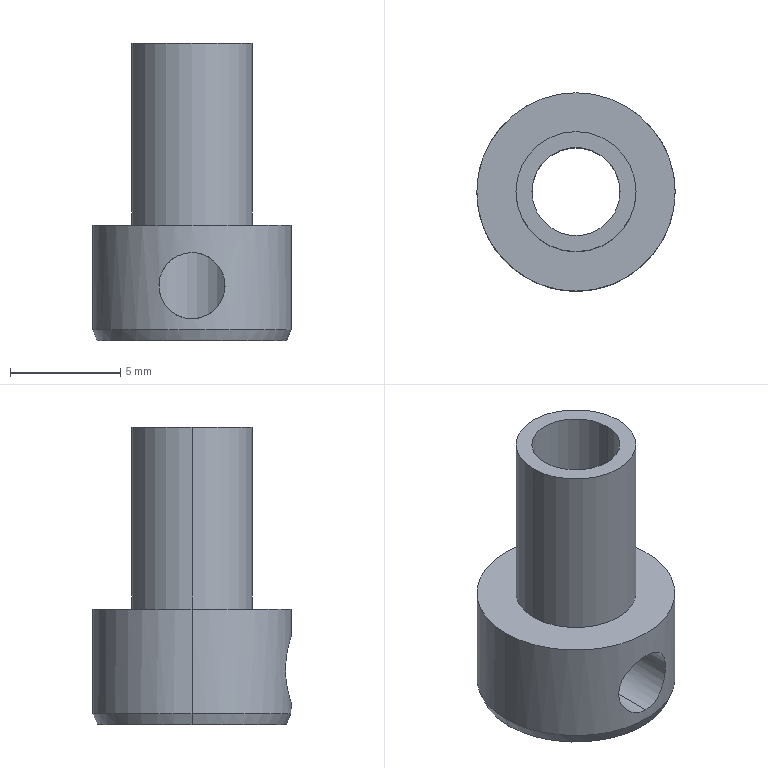Part | SolidWorks | features ICE 3, Blend 1, Extrusion 1 | 1 solid | 13 faces | box 9 x 9 x 13.5 mm | volume 337.082 mm3 | cylinder 8 | plane 3 | spline 2 | commonest cylinder face diameters 3 x2 4 x2 5.45 x2 9 x2
STEP:
#1=CARTESIAN_POINT('',(0.,-4.5,3.5));
#2=VERTEX_POINT('',#1);
#3=CARTESIAN_POINT('',(0.,-4.5,0.5));
#4=VERTEX_POINT('',#3);
#5=CARTESIAN_POINT('',(0.,-4.5,3.5));
#6=CARTESIAN_POINT('',(-0.09988,-4.5,3.5));
#7=CARTESIAN_POINT('',(-0.198,-4.497,3.49));
#8=CARTESIAN_POINT('',(-0.3907,-4.484,3.452));
#9=CARTESIAN_POINT('',(-0.4864,-4.475,3.422));
#10=CARTESIAN_POINT('',(-0.7584,-4.439,3.309));
#11=CARTESIAN_POINT('',(-0.9239,-4.406,3.198));
#12=CARTESIAN_POINT('',(-1.198,-4.34,2.923));
#13=CARTESIAN_POINT('',(-1.31,-4.306,2.757));
#14=CARTESIAN_POINT('',(-1.46,-4.257,2.396));
#15=CARTESIAN_POINT('',(-1.5,-4.243,2.198));
#16=CARTESIAN_POINT('',(-1.5,-4.243,1.902));
#17=CARTESIAN_POINT('',(-1.49,-4.246,1.802));
#18=CARTESIAN_POINT('',(-1.451,-4.26,1.609));
#19=CARTESIAN_POINT('',(-1.423,-4.269,1.515));
#20=CARTESIAN_POINT('',(-1.309,-4.306,1.241));
#21=CARTESIAN_POINT('',(-1.198,-4.34,1.077));
#22=CARTESIAN_POINT('',(-0.9912,-4.39,0.8699));
#23=CARTESIAN_POINT('',(-0.9162,-4.407,0.8083));
#24=CARTESIAN_POINT('',(-0.7541,-4.437,0.6997));
#25=CARTESIAN_POINT('',(-0.6663,-4.451,0.6526));
#26=CARTESIAN_POINT('',(-0.3954,-4.486,0.5399));
#27=CARTESIAN_POINT('',(-0.1968,-4.5,0.5));
#28=CARTESIAN_POINT('',(0.,-4.5,0.5));
#29=B_SPLINE_CURVE_WITH_KNOTS('',3,(#5,#6,#7,#8,#9,#10,#11,#12,#13,#14,#15,#16,#17,#18,#19,#20,#21,#22,#23,#24,#25,#26,#27,#28),.UNSPECIFIED.,.F.,.F.,(4,2,2,2,2,2,2,2,2,2,2,4),(0.,0.0002952,0.0005905,0.001181,0.001771,0.002362,0.002657,0.002952,0.003543,0.003838,0.004133,0.004724),.UNSPECIFIED.);
#30=EDGE_CURVE('',#2,#4,#29,.T.);
#31=ORIENTED_EDGE('',*,*,#30,.T.);
#32=CARTESIAN_POINT('',(0.,-2.,0.5));
#33=VERTEX_POINT('',#32);
#34=CARTESIAN_POINT('',(0.,-4.501,0.5));
#35=DIRECTION('',(0.,1.,0.));
#36=VECTOR('',#35,1000.);
#37=LINE('',#34,#36);
#38=EDGE_CURVE('',#4,#33,#37,.T.);
#39=ORIENTED_EDGE('',*,*,#38,.T.);
#40=CARTESIAN_POINT('',(0.,-2.,3.5));
#41=VERTEX_POINT('',#40);
#42=CARTESIAN_POINT('',(0.,-2.,0.5));
#43=CARTESIAN_POINT('',(-0.1025,-2.,0.5));
#44=CARTESIAN_POINT('',(-0.2067,-1.992,0.5108));
#45=CARTESIAN_POINT('',(-0.4052,-1.961,0.5522));
#46=CARTESIAN_POINT('',(-0.5023,-1.938,0.5831));
#47=CARTESIAN_POINT('',(-0.7754,-1.853,0.7007));
#48=CARTESIAN_POINT('',(-0.9353,-1.775,0.8124));
#49=CARTESIAN_POINT('',(-1.199,-1.608,1.079));
#50=CARTESIAN_POINT('',(-1.305,-1.519,1.237));
#51=CARTESIAN_POINT('',(-1.455,-1.376,1.589));
#52=CARTESIAN_POINT('',(-1.5,-1.323,1.794));
#53=CARTESIAN_POINT('',(-1.5,-1.323,2.207));
#54=CARTESIAN_POINT('',(-1.456,-1.375,2.409));
#55=CARTESIAN_POINT('',(-1.343,-1.483,2.675));
#56=CARTESIAN_POINT('',(-1.297,-1.524,2.759));
#57=CARTESIAN_POINT('',(-1.192,-1.607,2.915));
#58=CARTESIAN_POINT('',(-1.133,-1.65,2.987));
#59=CARTESIAN_POINT('',(-1.001,-1.733,3.121));
#60=CARTESIAN_POINT('',(-0.9275,-1.774,3.183));
#61=CARTESIAN_POINT('',(-0.7704,-1.848,3.291));
#62=CARTESIAN_POINT('',(-0.6862,-1.881,3.338));
#63=CARTESIAN_POINT('',(-0.4131,-1.966,3.456));
#64=CARTESIAN_POINT('',(-0.2077,-2.,3.5));
#65=CARTESIAN_POINT('',(0.,-2.,3.5));
#66=B_SPLINE_CURVE_WITH_KNOTS('',3,(#42,#43,#44,#45,#46,#47,#48,#49,#50,#51,#52,#53,#54,#55,#56,#57,#58,#59,#60,#61,#62,#63,#64,#65),.UNSPECIFIED.,.F.,.F.,(4,2,2,2,2,2,2,2,2,2,2,4),(0.004913,0.005219,0.005526,0.006139,0.006751,0.007364,0.007977,0.008283,0.00859,0.008896,0.009203,0.009816),.UNSPECIFIED.);
#67=EDGE_CURVE('',#33,#41,#66,.T.);
#68=ORIENTED_EDGE('',*,*,#67,.T.);
#69=CARTESIAN_POINT('',(0.,-4.501,3.5));
#70=DIRECTION('',(0.,1.,0.));
#71=VECTOR('',#70,1000.);
#72=LINE('',#69,#71);
#73=EDGE_CURVE('',#2,#41,#72,.T.);
#74=ORIENTED_EDGE('',*,*,#73,.F.);
#75=EDGE_LOOP('',(#31,#39,#68,#74));
#76=FACE_OUTER_BOUND('',#75,.T.);
#77=CARTESIAN_POINT('',(0.,-4.501,2.));
#78=DIRECTION('',(0.,1.,0.));
#79=DIRECTION('',(0.,0.,1.));
#80=AXIS2_PLACEMENT_3D('',#77,#78,#79);
#81=CYLINDRICAL_SURFACE('',#80,1.5);
#82=ADVANCED_FACE('',(#76),#81,.F.);
#83=CARTESIAN_POINT('',(0.,-2.,3.5));
#84=CARTESIAN_POINT('',(0.104,-2.,3.5));
#85=CARTESIAN_POINT('',(0.2056,-1.992,3.489));
#86=CARTESIAN_POINT('',(0.4043,-1.961,3.448));
#87=CARTESIAN_POINT('',(0.5019,-1.938,3.417));
#88=CARTESIAN_POINT('',(0.7741,-1.854,3.3));
#89=CARTESIAN_POINT('',(0.9344,-1.775,3.188));
#90=CARTESIAN_POINT('',(1.199,-1.608,2.921));
#91=CARTESIAN_POINT('',(1.305,-1.519,2.765));
#92=CARTESIAN_POINT('',(1.418,-1.411,2.498));
#93=CARTESIAN_POINT('',(1.448,-1.38,2.403));
#94=CARTESIAN_POINT('',(1.489,-1.335,2.207));
#95=CARTESIAN_POINT('',(1.5,-1.323,2.102));
#96=CARTESIAN_POINT('',(1.5,-1.323,1.898));
#97=CARTESIAN_POINT('',(1.489,-1.335,1.794));
#98=CARTESIAN_POINT('',(1.448,-1.38,1.596));
#99=CARTESIAN_POINT('',(1.418,-1.411,1.502));
#100=CARTESIAN_POINT('',(1.342,-1.484,1.324));
#101=CARTESIAN_POINT('',(1.297,-1.524,1.241));
#102=CARTESIAN_POINT('',(1.192,-1.607,1.085));
#103=CARTESIAN_POINT('',(1.132,-1.651,1.012));
#104=CARTESIAN_POINT('',(0.9999,-1.734,0.878));
#105=CARTESIAN_POINT('',(0.9277,-1.774,0.8174));
#106=CARTESIAN_POINT('',(0.7696,-1.848,0.7089));
#107=CARTESIAN_POINT('',(0.683,-1.882,0.6609));
#108=CARTESIAN_POINT('',(0.4107,-1.967,0.5438));
#109=CARTESIAN_POINT('',(0.2055,-2.,0.5));
#110=CARTESIAN_POINT('',(0.,-2.,0.5));
#111=B_SPLINE_CURVE_WITH_KNOTS('',3,(#83,#84,#85,#86,#87,#88,#89,#90,#91,#92,#93,#94,#95,#96,#97,#98,#99,#100,#101,#102,#103,#104,#105,#106,#107,#108,#109,#110),.UNSPECIFIED.,.F.,.F.,(4,2,2,2,2,2,2,2,2,2,2,2,2,4),(0.,0.0003071,0.0006141,0.001228,0.001842,0.002149,0.002456,0.002764,0.003071,0.003378,0.003685,0.003992,0.004299,0.004913),.UNSPECIFIED.);
#112=EDGE_CURVE('',#41,#33,#111,.T.);
#113=ORIENTED_EDGE('',*,*,#112,.F.);
#114=ORIENTED_EDGE('',*,*,#67,.F.);
#115=EDGE_LOOP('',(#113,#114));
#116=FACE_BOUND('',#115,.T.);
#117=CARTESIAN_POINT('',(2.,0.,-0.5));
#118=VERTEX_POINT('',#117);
#119=CARTESIAN_POINT('',(-2.,0.,-0.5));
#120=VERTEX_POINT('',#119);
#121=CARTESIAN_POINT('',(0.,0.,-0.5));
#122=DIRECTION('',(0.,0.,-1.));
#123=DIRECTION('',(-1.,0.,0.));
#124=AXIS2_PLACEMENT_3D('',#121,#122,#123);
#125=CIRCLE('',#124,2.);
#126=EDGE_CURVE('',#118,#120,#125,.T.);
#127=ORIENTED_EDGE('',*,*,#126,.T.);
#128=CARTESIAN_POINT('',(-2.,0.,13.));
#129=VERTEX_POINT('',#128);
#130=CARTESIAN_POINT('',(-2.,0.,-0.511));
#131=DIRECTION('',(0.,0.,1.));
#132=VECTOR('',#131,1000.);
#133=LINE('',#130,#132);
#134=EDGE_CURVE('',#120,#129,#133,.T.);
#135=ORIENTED_EDGE('',*,*,#134,.T.);
#136=CARTESIAN_POINT('',(2.,0.,13.));
#137=VERTEX_POINT('',#136);
#138=CARTESIAN_POINT('',(0.,0.,13.));
#139=DIRECTION('',(0.,0.,1.));
#140=DIRECTION('',(1.,0.,0.));
#141=AXIS2_PLACEMENT_3D('',#138,#139,#140);
#142=CIRCLE('',#141,2.);
#143=EDGE_CURVE('',#129,#137,#142,.T.);
#144=ORIENTED_EDGE('',*,*,#143,.T.);
#145=CARTESIAN_POINT('',(2.,0.,-0.511));
#146=DIRECTION('',(0.,0.,1.));
#147=VECTOR('',#146,1000.);
#148=LINE('',#145,#147);
#149=EDGE_CURVE('',#118,#137,#148,.T.);
#150=ORIENTED_EDGE('',*,*,#149,.F.);
#151=EDGE_LOOP('',(#127,#135,#144,#150));
#152=FACE_OUTER_BOUND('',#151,.T.);
#153=CARTESIAN_POINT('',(0.,0.,-0.511));
#154=DIRECTION('',(0.,0.,1.));
#155=DIRECTION('',(1.,0.,0.));
#156=AXIS2_PLACEMENT_3D('',#153,#154,#155);
#157=CYLINDRICAL_SURFACE('',#156,2.);
#158=ADVANCED_FACE('',(#116,#152),#157,.F.);
#159=CARTESIAN_POINT('',(2.725,0.,4.75));
#160=VERTEX_POINT('',#159);
#161=CARTESIAN_POINT('',(-2.725,0.,4.75));
#162=VERTEX_POINT('',#161);
#163=CARTESIAN_POINT('',(0.,0.,4.75));
#164=DIRECTION('',(0.,0.,1.));
#165=DIRECTION('',(1.,0.,0.));
#166=AXIS2_PLACEMENT_3D('',#163,#164,#165);
#167=CIRCLE('',#166,2.725);
#168=EDGE_CURVE('',#160,#162,#167,.T.);
#169=ORIENTED_EDGE('',*,*,#168,.T.);
#170=CARTESIAN_POINT('',(-2.725,0.,13.));
#171=VERTEX_POINT('',#170);
#172=CARTESIAN_POINT('',(-2.725,0.,4.75));
#173=DIRECTION('',(0.,0.,1.));
#174=VECTOR('',#173,1000.);
#175=LINE('',#172,#174);
#176=EDGE_CURVE('',#162,#171,#175,.T.);
#177=ORIENTED_EDGE('',*,*,#176,.T.);
#178=CARTESIAN_POINT('',(2.725,0.,13.));
#179=VERTEX_POINT('',#178);
#180=CARTESIAN_POINT('',(0.,0.,13.));
#181=DIRECTION('',(0.,0.,1.));
#182=DIRECTION('',(1.,0.,0.));
#183=AXIS2_PLACEMENT_3D('',#180,#181,#182);
#184=CIRCLE('',#183,2.725);
#185=EDGE_CURVE('',#179,#171,#184,.T.);
#186=ORIENTED_EDGE('',*,*,#185,.F.);
#187=CARTESIAN_POINT('',(2.725,0.,4.75));
#188=DIRECTION('',(0.,0.,1.));
#189=VECTOR('',#188,1000.);
#190=LINE('',#187,#189);
#191=EDGE_CURVE('',#160,#179,#190,.T.);
#192=ORIENTED_EDGE('',*,*,#191,.F.);
#193=EDGE_LOOP('',(#169,#177,#186,#192));
#194=FACE_OUTER_BOUND('',#193,.T.);
#195=CARTESIAN_POINT('',(0.,0.,4.75));
#196=DIRECTION('',(0.,0.,1.));
#197=DIRECTION('',(1.,0.,0.));
#198=AXIS2_PLACEMENT_3D('',#195,#196,#197);
#199=CYLINDRICAL_SURFACE('',#198,2.725);
#200=ADVANCED_FACE('',(#194),#199,.T.);
#201=CARTESIAN_POINT('',(-4.3,0.,-0.5));
#202=VERTEX_POINT('',#201);
#203=CARTESIAN_POINT('',(4.3,0.,-0.5));
#204=VERTEX_POINT('',#203);
#205=CARTESIAN_POINT('',(0.,0.,-0.5));
#206=DIRECTION('',(0.,0.,-1.));
#207=DIRECTION('',(-1.,0.,0.));
#208=AXIS2_PLACEMENT_3D('',#205,#206,#207);
#209=CIRCLE('',#208,4.3);
#210=EDGE_CURVE('',#202,#204,#209,.T.);
#211=ORIENTED_EDGE('',*,*,#210,.F.);
#212=CARTESIAN_POINT('',(-4.5,0.,0.));
#213=VERTEX_POINT('',#212);
#214=CARTESIAN_POINT('',(-4.3,0.,-0.5));
#215=CARTESIAN_POINT('',(-4.367,0.,-0.3333));
#216=CARTESIAN_POINT('',(-4.433,0.,-0.1667));
#217=CARTESIAN_POINT('',(-4.5,0.,0.));
#218=B_SPLINE_CURVE_WITH_KNOTS('',3,(#214,#215,#216,#217),.UNSPECIFIED.,.F.,.F.,(4,4),(0.,1.),.UNSPECIFIED.);
#219=EDGE_CURVE('',#202,#213,#218,.T.);
#220=ORIENTED_EDGE('',*,*,#219,.T.);
#221=CARTESIAN_POINT('',(4.5,0.,0.));
#222=VERTEX_POINT('',#221);
#223=CARTESIAN_POINT('',(-4.5,0.,0.));
#224=CARTESIAN_POINT('',(-4.5,0.2973,0.));
#225=CARTESIAN_POINT('',(-4.471,0.5901,-0.001205));
#226=CARTESIAN_POINT('',(-4.356,1.167,-0.002331));
#227=CARTESIAN_POINT('',(-4.269,1.454,-0.00232));
#228=CARTESIAN_POINT('',(-4.043,1.997,-0.001168));
#229=CARTESIAN_POINT('',(-3.905,2.255,-0.000117));
#230=CARTESIAN_POINT('',(-3.577,2.746,0.001603));
#231=CARTESIAN_POINT('',(-3.388,2.976,0.002209));
#232=CARTESIAN_POINT('',(-2.973,3.391,0.002204));
#233=CARTESIAN_POINT('',(-2.746,3.578,0.001602));
#234=CARTESIAN_POINT('',(-2.252,3.908,-0.000131));
#235=CARTESIAN_POINT('',(-1.992,4.046,-0.001182));
#236=CARTESIAN_POINT('',(-1.451,4.27,-0.002322));
#237=CARTESIAN_POINT('',(-1.165,4.357,-0.002329));
#238=CARTESIAN_POINT('',(-0.5863,4.471,-0.001194));
#239=CARTESIAN_POINT('',(-0.2946,4.5,-0.000001214));
#240=CARTESIAN_POINT('',(0.2938,4.5,0.000001212));
#241=CARTESIAN_POINT('',(0.5919,4.471,-0.001209));
#242=CARTESIAN_POINT('',(1.167,4.356,-0.00233));
#243=CARTESIAN_POINT('',(1.448,4.271,-0.002327));
#244=CARTESIAN_POINT('',(1.995,4.044,-0.001175));
#245=CARTESIAN_POINT('',(2.257,3.904,-0.0001123));
#246=CARTESIAN_POINT('',(2.744,3.579,0.001596));
#247=CARTESIAN_POINT('',(2.974,3.39,0.002208));
#248=CARTESIAN_POINT('',(3.392,2.972,0.002205));
#249=CARTESIAN_POINT('',(3.578,2.745,0.001599));
#250=CARTESIAN_POINT('',(3.904,2.257,-0.0001112));
#251=CARTESIAN_POINT('',(4.045,1.993,-0.001181));
#252=CARTESIAN_POINT('',(4.27,1.449,-0.002324));
#253=CARTESIAN_POINT('',(4.356,1.169,-0.002333));
#254=CARTESIAN_POINT('',(4.471,0.5903,-0.001206));
#255=CARTESIAN_POINT('',(4.5,0.2932,0.));
#256=CARTESIAN_POINT('',(4.5,0.,0.));
#257=B_SPLINE_CURVE_WITH_KNOTS('',3,(#223,#224,#225,#226,#227,#228,#229,#230,#231,#232,#233,#234,#235,#236,#237,#238,#239,#240,#241,#242,#243,#244,#245,#246,#247,#248,#249,#250,#251,#252,#253,#254,#255,#256),.UNSPECIFIED.,.F.,.F.,(4,2,2,2,2,2,2,2,2,2,2,2,2,2,2,2,4),(0.,0.0008817,0.001763,0.002645,0.003527,0.004409,0.00529,0.006172,0.007054,0.007936,0.008817,0.009699,0.01058,0.01146,0.01234,0.01323,0.01411),.UNSPECIFIED.);
#258=EDGE_CURVE('',#213,#222,#257,.T.);
#259=ORIENTED_EDGE('',*,*,#258,.T.);
#260=CARTESIAN_POINT('',(4.3,0.,-0.5));
#261=CARTESIAN_POINT('',(4.367,0.,-0.3333));
#262=CARTESIAN_POINT('',(4.433,0.,-0.1667));
#263=CARTESIAN_POINT('',(4.5,0.,0.));
#264=B_SPLINE_CURVE_WITH_KNOTS('',3,(#260,#261,#262,#263),.UNSPECIFIED.,.F.,.F.,(4,4),(0.,1.),.UNSPECIFIED.);
#265=EDGE_CURVE('',#204,#222,#264,.T.);
#266=ORIENTED_EDGE('',*,*,#265,.F.);
#267=EDGE_LOOP('',(#211,#220,#259,#266));
#268=FACE_OUTER_BOUND('',#267,.T.);
#269=CARTESIAN_POINT('',(4.3,0.,-0.5));
#270=CARTESIAN_POINT('',(4.367,0.,-0.3333));
#271=CARTESIAN_POINT('',(4.433,0.,-0.1667));
#272=CARTESIAN_POINT('',(4.5,0.,0.));
#273=CARTESIAN_POINT('',(4.501,0.,0.0019));
#274=CARTESIAN_POINT('',(4.502,0.,0.0038));
#275=CARTESIAN_POINT('',(4.502,0.,0.0057));
#276=CARTESIAN_POINT('',(4.3,0.1187,-0.5));
#277=CARTESIAN_POINT('',(4.367,0.1205,-0.3333));
#278=CARTESIAN_POINT('',(4.433,0.1223,-0.1667));
#279=CARTESIAN_POINT('',(4.5,0.1242,0.));
#280=CARTESIAN_POINT('',(4.501,0.1242,0.0019));
#281=CARTESIAN_POINT('',(4.502,0.1242,0.0038));
#282=CARTESIAN_POINT('',(4.502,0.1242,0.0057));
#283=CARTESIAN_POINT('',(4.29,0.3538,-0.5));
#284=CARTESIAN_POINT('',(4.357,0.3592,-0.3333));
#285=CARTESIAN_POINT('',(4.423,0.3647,-0.1667));
#286=CARTESIAN_POINT('',(4.49,0.3702,0.));
#287=CARTESIAN_POINT('',(4.491,0.3703,0.0019));
#288=CARTESIAN_POINT('',(4.491,0.3703,0.0038));
#289=CARTESIAN_POINT('',(4.492,0.3704,0.0057));
#290=CARTESIAN_POINT('',(4.248,0.6986,-0.5));
#291=CARTESIAN_POINT('',(4.314,0.7094,-0.3333));
#292=CARTESIAN_POINT('',(4.38,0.7202,-0.1667));
#293=CARTESIAN_POINT('',(4.446,0.7311,0.));
#294=CARTESIAN_POINT('',(4.446,0.7312,0.0019));
#295=CARTESIAN_POINT('',(4.447,0.7313,0.0038));
#296=CARTESIAN_POINT('',(4.448,0.7314,0.0057));
#297=CARTESIAN_POINT('',(4.179,1.034,-0.5));
#298=CARTESIAN_POINT('',(4.244,1.051,-0.3333));
#299=CARTESIAN_POINT('',(4.309,1.067,-0.1667));
#300=CARTESIAN_POINT('',(4.374,1.083,0.));
#301=CARTESIAN_POINT('',(4.374,1.083,0.0019));
#302=CARTESIAN_POINT('',(4.375,1.083,0.0038));
#303=CARTESIAN_POINT('',(4.376,1.083,0.0057));
#304=CARTESIAN_POINT('',(3.612,2.99,-0.5));
#305=CARTESIAN_POINT('',(3.668,3.036,-0.3333));
#306=CARTESIAN_POINT('',(3.724,3.083,-0.1667));
#307=CARTESIAN_POINT('',(3.78,3.129,0.));
#308=CARTESIAN_POINT('',(3.781,3.129,0.0019));
#309=CARTESIAN_POINT('',(3.782,3.13,0.0038));
#310=CARTESIAN_POINT('',(3.782,3.13,0.0057));
#311=CARTESIAN_POINT('',(1.899,4.3,-0.5));
#312=CARTESIAN_POINT('',(1.928,4.367,-0.3333));
#313=CARTESIAN_POINT('',(1.957,4.433,-0.1667));
#314=CARTESIAN_POINT('',(1.987,4.5,0.));
#315=CARTESIAN_POINT('',(1.987,4.501,0.0019));
#316=CARTESIAN_POINT('',(1.988,4.502,0.0038));
#317=CARTESIAN_POINT('',(1.988,4.502,0.0057));
#318=CARTESIAN_POINT('',(-2.373,4.3,-0.5));
#319=CARTESIAN_POINT('',(-2.41,4.367,-0.3333));
#320=CARTESIAN_POINT('',(-2.447,4.433,-0.1667));
#321=CARTESIAN_POINT('',(-2.484,4.5,0.));
#322=CARTESIAN_POINT('',(-2.484,4.501,0.0019));
#323=CARTESIAN_POINT('',(-2.484,4.502,0.0038));
#324=CARTESIAN_POINT('',(-2.485,4.502,0.0057));
#325=CARTESIAN_POINT('',(-4.3,2.373,-0.5));
#326=CARTESIAN_POINT('',(-4.367,2.41,-0.3333));
#327=CARTESIAN_POINT('',(-4.433,2.447,-0.1667));
#328=CARTESIAN_POINT('',(-4.5,2.484,0.));
#329=CARTESIAN_POINT('',(-4.501,2.484,0.0019));
#330=CARTESIAN_POINT('',(-4.502,2.484,0.0038));
#331=CARTESIAN_POINT('',(-4.502,2.485,0.0057));
#332=CARTESIAN_POINT('',(-4.3,-2.373,-0.5));
#333=CARTESIAN_POINT('',(-4.367,-2.41,-0.3333));
#334=CARTESIAN_POINT('',(-4.433,-2.447,-0.1667));
#335=CARTESIAN_POINT('',(-4.5,-2.484,0.));
#336=CARTESIAN_POINT('',(-4.501,-2.484,0.0019));
#337=CARTESIAN_POINT('',(-4.502,-2.484,0.0038));
#338=CARTESIAN_POINT('',(-4.502,-2.485,0.0057));
#339=CARTESIAN_POINT('',(-2.373,-4.3,-0.5));
#340=CARTESIAN_POINT('',(-2.41,-4.367,-0.3333));
#341=CARTESIAN_POINT('',(-2.447,-4.433,-0.1667));
#342=CARTESIAN_POINT('',(-2.484,-4.5,0.));
#343=CARTESIAN_POINT('',(-2.484,-4.501,0.0019));
#344=CARTESIAN_POINT('',(-2.484,-4.502,0.0038));
#345=CARTESIAN_POINT('',(-2.485,-4.502,0.0057));
#346=CARTESIAN_POINT('',(1.899,-4.3,-0.5));
#347=CARTESIAN_POINT('',(1.928,-4.367,-0.3333));
#348=CARTESIAN_POINT('',(1.957,-4.433,-0.1667));
#349=CARTESIAN_POINT('',(1.987,-4.5,0.));
#350=CARTESIAN_POINT('',(1.987,-4.501,0.0019));
#351=CARTESIAN_POINT('',(1.988,-4.502,0.0038));
#352=CARTESIAN_POINT('',(1.988,-4.502,0.0057));
#353=CARTESIAN_POINT('',(3.612,-2.99,-0.5));
#354=CARTESIAN_POINT('',(3.668,-3.036,-0.3333));
#355=CARTESIAN_POINT('',(3.724,-3.083,-0.1667));
#356=CARTESIAN_POINT('',(3.78,-3.129,0.));
#357=CARTESIAN_POINT('',(3.781,-3.129,0.0019));
#358=CARTESIAN_POINT('',(3.782,-3.13,0.0038));
#359=CARTESIAN_POINT('',(3.782,-3.13,0.0057));
#360=CARTESIAN_POINT('',(4.179,-1.034,-0.5));
#361=CARTESIAN_POINT('',(4.244,-1.051,-0.3333));
#362=CARTESIAN_POINT('',(4.309,-1.067,-0.1667));
#363=CARTESIAN_POINT('',(4.374,-1.083,0.));
#364=CARTESIAN_POINT('',(4.374,-1.083,0.0019));
#365=CARTESIAN_POINT('',(4.375,-1.083,0.0038));
#366=CARTESIAN_POINT('',(4.376,-1.083,0.0057));
#367=CARTESIAN_POINT('',(4.248,-0.6986,-0.5));
#368=CARTESIAN_POINT('',(4.314,-0.7094,-0.3333));
#369=CARTESIAN_POINT('',(4.38,-0.7202,-0.1667));
#370=CARTESIAN_POINT('',(4.446,-0.7311,0.));
#371=CARTESIAN_POINT('',(4.446,-0.7312,0.0019));
#372=CARTESIAN_POINT('',(4.447,-0.7313,0.0038));
#373=CARTESIAN_POINT('',(4.448,-0.7314,0.0057));
#374=CARTESIAN_POINT('',(4.29,-0.3538,-0.5));
#375=CARTESIAN_POINT('',(4.357,-0.3592,-0.3333));
#376=CARTESIAN_POINT('',(4.423,-0.3647,-0.1667));
#377=CARTESIAN_POINT('',(4.49,-0.3702,0.));
#378=CARTESIAN_POINT('',(4.491,-0.3703,0.0019));
#379=CARTESIAN_POINT('',(4.491,-0.3703,0.0038));
#380=CARTESIAN_POINT('',(4.492,-0.3704,0.0057));
#381=CARTESIAN_POINT('',(4.3,-0.1187,-0.5));
#382=CARTESIAN_POINT('',(4.367,-0.1205,-0.3333));
#383=CARTESIAN_POINT('',(4.433,-0.1223,-0.1667));
#384=CARTESIAN_POINT('',(4.5,-0.1242,0.));
#385=CARTESIAN_POINT('',(4.501,-0.1242,0.0019));
#386=CARTESIAN_POINT('',(4.502,-0.1242,0.0038));
#387=CARTESIAN_POINT('',(4.502,-0.1242,0.0057));
#388=CARTESIAN_POINT('',(4.3,0.,-0.5));
#389=CARTESIAN_POINT('',(4.367,0.,-0.3333));
#390=CARTESIAN_POINT('',(4.433,0.,-0.1667));
#391=CARTESIAN_POINT('',(4.5,0.,0.));
#392=CARTESIAN_POINT('',(4.501,0.,0.0019));
#393=CARTESIAN_POINT('',(4.502,0.,0.0038));
#394=CARTESIAN_POINT('',(4.502,0.,0.0057));
#395=B_SPLINE_SURFACE_WITH_KNOTS('',3,3,((#269,#270,#271,#272,#273,#274,#275),(#276,#277,#278,#279,#280,#281,#282),(#283,#284,#285,#286,#287,#288,#289),(#290,#291,#292,#293,#294,#295,#296),(#297,#298,#299,#300,#301,#302,#303),(#304,#305,#306,#307,#308,#309,#310),(#311,#312,#313,#314,#315,#316,#317),(#318,#319,#320,#321,#322,#323,#324),(#325,#326,#327,#328,#329,#330,#331),(#332,#333,#334,#335,#336,#337,#338),(#339,#340,#341,#342,#343,#344,#345),(#346,#347,#348,#349,#350,#351,#352),(#353,#354,#355,#356,#357,#358,#359),(#360,#361,#362,#363,#364,#365,#366),(#367,#368,#369,#370,#371,#372,#373),(#374,#375,#376,#377,#378,#379,#380),(#381,#382,#383,#384,#385,#386,#387),(#388,#389,#390,#391,#392,#393,#394)),.UNSPECIFIED.,.T.,.F.,.F.,(4,1,1,1,1,2,2,2,1,1,1,1,4),(4,3,4),(0.,0.0125,0.025,0.0375,0.05,0.25,0.5,0.75,0.95,0.9625,0.975,0.9875,1.),(0.,1.,1.011),.UNSPECIFIED.);
#396=ADVANCED_FACE('',(#268),#395,.T.);
#397=CARTESIAN_POINT('',(4.5,0.,4.75));
#398=VERTEX_POINT('',#397);
#399=CARTESIAN_POINT('',(-4.5,0.,4.75));
#400=VERTEX_POINT('',#399);
#401=CARTESIAN_POINT('',(0.,0.,4.75));
#402=DIRECTION('',(0.,0.,1.));
#403=DIRECTION('',(1.,0.,0.));
#404=AXIS2_PLACEMENT_3D('',#401,#402,#403);
#405=CIRCLE('',#404,4.5);
#406=EDGE_CURVE('',#398,#400,#405,.T.);
#407=ORIENTED_EDGE('',*,*,#406,.F.);
#408=CARTESIAN_POINT('',(4.5,0.,13.));
#409=DIRECTION('',(0.,0.,-1.));
#410=VECTOR('',#409,1000.);
#411=LINE('',#408,#410);
#412=EDGE_CURVE('',#398,#222,#411,.T.);
#413=ORIENTED_EDGE('',*,*,#412,.T.);
#414=ORIENTED_EDGE('',*,*,#258,.F.);
#415=CARTESIAN_POINT('',(-4.5,0.,13.));
#416=DIRECTION('',(0.,0.,-1.));
#417=VECTOR('',#416,1000.);
#418=LINE('',#415,#417);
#419=EDGE_CURVE('',#400,#213,#418,.T.);
#420=ORIENTED_EDGE('',*,*,#419,.F.);
#421=EDGE_LOOP('',(#407,#413,#414,#420));
#422=FACE_OUTER_BOUND('',#421,.T.);
#423=CARTESIAN_POINT('',(0.,0.,13.));
#424=DIRECTION('',(0.,0.,-1.));
#425=DIRECTION('',(-1.,0.,0.));
#426=AXIS2_PLACEMENT_3D('',#423,#424,#425);
#427=CYLINDRICAL_SURFACE('',#426,4.5);
#428=ADVANCED_FACE('',(#422),#427,.T.);
#429=ORIENTED_EDGE('',*,*,#412,.F.);
#430=CARTESIAN_POINT('',(0.,0.,4.75));
#431=DIRECTION('',(0.,0.,1.));
#432=DIRECTION('',(1.,0.,0.));
#433=AXIS2_PLACEMENT_3D('',#430,#431,#432);
#434=CIRCLE('',#433,4.5);
#435=EDGE_CURVE('',#400,#398,#434,.T.);
#436=ORIENTED_EDGE('',*,*,#435,.F.);
#437=ORIENTED_EDGE('',*,*,#419,.T.);
#438=CARTESIAN_POINT('',(4.5,0.,0.));
#439=CARTESIAN_POINT('',(4.5,-0.2932,0.));
#440=CARTESIAN_POINT('',(4.472,-0.5855,-0.001194));
#441=CARTESIAN_POINT('',(4.356,-1.169,-0.002335));
#442=CARTESIAN_POINT('',(4.27,-1.45,-0.002323));
#443=CARTESIAN_POINT('',(4.046,-1.991,-0.001185));
#444=CARTESIAN_POINT('',(3.905,-2.255,-0.0001189));
#445=CARTESIAN_POINT('',(3.578,-2.745,0.0016));
#446=CARTESIAN_POINT('',(3.392,-2.972,0.002203));
#447=CARTESIAN_POINT('',(2.976,-3.388,0.00221));
#448=CARTESIAN_POINT('',(2.745,-3.578,0.001598));
#449=CARTESIAN_POINT('',(2.257,-3.904,-0.0001119));
#450=CARTESIAN_POINT('',(1.998,-4.043,-0.001165));
#451=CARTESIAN_POINT('',(1.452,-4.27,-0.002324));
#452=CARTESIAN_POINT('',(1.168,-4.356,-0.00233));
#453=CARTESIAN_POINT('',(0.5929,-4.47,-0.001212));
#454=CARTESIAN_POINT('',(0.298,-4.5,-0.000006023));
#455=CARTESIAN_POINT('',(-0.2942,-4.5,0.000005984));
#456=CARTESIAN_POINT('',(-0.5861,-4.471,-0.001192));
#457=CARTESIAN_POINT('',(-1.162,-4.357,-0.002325));
#458=CARTESIAN_POINT('',(-1.448,-4.271,-0.002325));
#459=CARTESIAN_POINT('',(-1.992,-4.046,-0.001183));
#460=CARTESIAN_POINT('',(-2.251,-3.908,-0.0001348));
#461=CARTESIAN_POINT('',(-2.741,-3.581,0.001587));
#462=CARTESIAN_POINT('',(-2.972,-3.391,0.002202));
#463=CARTESIAN_POINT('',(-3.387,-2.977,0.00221));
#464=CARTESIAN_POINT('',(-3.574,-2.75,0.001617));
#465=CARTESIAN_POINT('',(-3.904,-2.257,-0.0001101));
#466=CARTESIAN_POINT('',(-4.043,-1.997,-0.001165));
#467=CARTESIAN_POINT('',(-4.268,-1.456,-0.002317));
#468=CARTESIAN_POINT('',(-4.355,-1.171,-0.002336));
#469=CARTESIAN_POINT('',(-4.471,-0.5909,-0.001209));
#470=CARTESIAN_POINT('',(-4.5,-0.2973,0.));
#471=CARTESIAN_POINT('',(-4.5,0.,0.));
#472=B_SPLINE_CURVE_WITH_KNOTS('',3,(#438,#439,#440,#441,#442,#443,#444,#445,#446,#447,#448,#449,#450,#451,#452,#453,#454,#455,#456,#457,#458,#459,#460,#461,#462,#463,#464,#465,#466,#467,#468,#469,#470,#471),.UNSPECIFIED.,.F.,.F.,(4,2,2,2,2,2,2,2,2,2,2,2,2,2,2,2,4),(0.01411,0.01499,0.01587,0.01675,0.01763,0.01852,0.0194,0.02028,0.02116,0.02204,0.02292,0.02381,0.02469,0.02557,0.02645,0.02733,0.02821),.UNSPECIFIED.);
#473=EDGE_CURVE('',#222,#213,#472,.T.);
#474=ORIENTED_EDGE('',*,*,#473,.F.);
#475=EDGE_LOOP('',(#429,#436,#437,#474));
#476=FACE_OUTER_BOUND('',#475,.T.);
#477=ORIENTED_EDGE('',*,*,#30,.F.);
#478=CARTESIAN_POINT('',(0.,-4.5,0.5));
#479=CARTESIAN_POINT('',(0.1967,-4.5,0.5));
#480=CARTESIAN_POINT('',(0.3953,-4.486,0.5398));
#481=CARTESIAN_POINT('',(0.6668,-4.451,0.6528));
#482=CARTESIAN_POINT('',(0.7546,-4.437,0.6999));
#483=CARTESIAN_POINT('',(0.9165,-4.406,0.8086));
#484=CARTESIAN_POINT('',(0.9916,-4.39,0.8703));
#485=CARTESIAN_POINT('',(1.199,-4.34,1.078));
#486=CARTESIAN_POINT('',(1.309,-4.306,1.242));
#487=CARTESIAN_POINT('',(1.423,-4.269,1.515));
#488=CARTESIAN_POINT('',(1.451,-4.26,1.609));
#489=CARTESIAN_POINT('',(1.49,-4.246,1.801));
#490=CARTESIAN_POINT('',(1.5,-4.243,1.901));
#491=CARTESIAN_POINT('',(1.5,-4.243,2.099));
#492=CARTESIAN_POINT('',(1.49,-4.246,2.197));
#493=CARTESIAN_POINT('',(1.452,-4.259,2.391));
#494=CARTESIAN_POINT('',(1.422,-4.269,2.486));
#495=CARTESIAN_POINT('',(1.31,-4.306,2.757));
#496=CARTESIAN_POINT('',(1.198,-4.34,2.923));
#497=CARTESIAN_POINT('',(0.9921,-4.39,3.129));
#498=CARTESIAN_POINT('',(0.9155,-4.407,3.192));
#499=CARTESIAN_POINT('',(0.7534,-4.437,3.301));
#500=CARTESIAN_POINT('',(0.6676,-4.451,3.347));
#501=CARTESIAN_POINT('',(0.4863,-4.475,3.422));
#502=CARTESIAN_POINT('',(0.3906,-4.484,3.452));
#503=CARTESIAN_POINT('',(0.198,-4.497,3.49));
#504=CARTESIAN_POINT('',(0.09985,-4.5,3.5));
#505=CARTESIAN_POINT('',(0.,-4.5,3.5));
#506=B_SPLINE_CURVE_WITH_KNOTS('',3,(#478,#479,#480,#481,#482,#483,#484,#485,#486,#487,#488,#489,#490,#491,#492,#493,#494,#495,#496,#497,#498,#499,#500,#501,#502,#503,#504,#505),.UNSPECIFIED.,.F.,.F.,(4,2,2,2,2,2,2,2,2,2,2,2,2,4),(0.004724,0.005314,0.005609,0.005904,0.006495,0.00679,0.007085,0.00738,0.007675,0.008266,0.008561,0.008856,0.009151,0.009446),.UNSPECIFIED.);
#507=EDGE_CURVE('',#4,#2,#506,.T.);
#508=ORIENTED_EDGE('',*,*,#507,.F.);
#509=EDGE_LOOP('',(#477,#508));
#510=FACE_BOUND('',#509,.T.);
#511=CARTESIAN_POINT('',(0.,0.,13.));
#512=DIRECTION('',(0.,0.,-1.));
#513=DIRECTION('',(-1.,0.,0.));
#514=AXIS2_PLACEMENT_3D('',#511,#512,#513);
#515=CYLINDRICAL_SURFACE('',#514,4.5);
#516=ADVANCED_FACE('',(#476,#510),#515,.T.);
#517=ORIENTED_EDGE('',*,*,#126,.F.);
#518=CARTESIAN_POINT('',(0.,0.,-0.5));
#519=DIRECTION('',(0.,0.,-1.));
#520=DIRECTION('',(-1.,0.,0.));
#521=AXIS2_PLACEMENT_3D('',#518,#519,#520);
#522=CIRCLE('',#521,2.);
#523=EDGE_CURVE('',#120,#118,#522,.T.);
#524=ORIENTED_EDGE('',*,*,#523,.F.);
#525=EDGE_LOOP('',(#517,#524));
#526=FACE_BOUND('',#525,.T.);
#527=CARTESIAN_POINT('',(0.,0.,-0.5));
#528=DIRECTION('',(0.,0.,-1.));
#529=DIRECTION('',(-1.,0.,0.));
#530=AXIS2_PLACEMENT_3D('',#527,#528,#529);
#531=CIRCLE('',#530,4.3);
#532=EDGE_CURVE('',#204,#202,#531,.T.);
#533=ORIENTED_EDGE('',*,*,#532,.T.);
#534=ORIENTED_EDGE('',*,*,#210,.T.);
#535=EDGE_LOOP('',(#533,#534));
#536=FACE_OUTER_BOUND('',#535,.T.);
#537=CARTESIAN_POINT('',(0.,0.,-0.5));
#538=DIRECTION('',(0.,0.,-1.));
#539=DIRECTION('',(-1.,0.,0.));
#540=AXIS2_PLACEMENT_3D('',#537,#538,#539);
#541=PLANE('',#540);
#542=ADVANCED_FACE('',(#526,#536),#541,.T.);
#543=ORIENTED_EDGE('',*,*,#219,.F.);
#544=ORIENTED_EDGE('',*,*,#532,.F.);
#545=ORIENTED_EDGE('',*,*,#265,.T.);
#546=ORIENTED_EDGE('',*,*,#473,.T.);
#547=EDGE_LOOP('',(#543,#544,#545,#546));
#548=FACE_OUTER_BOUND('',#547,.T.);
#549=CARTESIAN_POINT('',(4.3,0.,-0.5));
#550=CARTESIAN_POINT('',(4.367,0.,-0.3333));
#551=CARTESIAN_POINT('',(4.433,0.,-0.1667));
#552=CARTESIAN_POINT('',(4.5,0.,0.));
#553=CARTESIAN_POINT('',(4.501,0.,0.0019));
#554=CARTESIAN_POINT('',(4.502,0.,0.0038));
#555=CARTESIAN_POINT('',(4.502,0.,0.0057));
#556=CARTESIAN_POINT('',(4.3,0.1187,-0.5));
#557=CARTESIAN_POINT('',(4.367,0.1205,-0.3333));
#558=CARTESIAN_POINT('',(4.433,0.1223,-0.1667));
#559=CARTESIAN_POINT('',(4.5,0.1242,0.));
#560=CARTESIAN_POINT('',(4.501,0.1242,0.0019));
#561=CARTESIAN_POINT('',(4.502,0.1242,0.0038));
#562=CARTESIAN_POINT('',(4.502,0.1242,0.0057));
#563=CARTESIAN_POINT('',(4.29,0.3538,-0.5));
#564=CARTESIAN_POINT('',(4.357,0.3592,-0.3333));
#565=CARTESIAN_POINT('',(4.423,0.3647,-0.1667));
#566=CARTESIAN_POINT('',(4.49,0.3702,0.));
#567=CARTESIAN_POINT('',(4.491,0.3703,0.0019));
#568=CARTESIAN_POINT('',(4.491,0.3703,0.0038));
#569=CARTESIAN_POINT('',(4.492,0.3704,0.0057));
#570=CARTESIAN_POINT('',(4.248,0.6986,-0.5));
#571=CARTESIAN_POINT('',(4.314,0.7094,-0.3333));
#572=CARTESIAN_POINT('',(4.38,0.7202,-0.1667));
#573=CARTESIAN_POINT('',(4.446,0.7311,0.));
#574=CARTESIAN_POINT('',(4.446,0.7312,0.0019));
#575=CARTESIAN_POINT('',(4.447,0.7313,0.0038));
#576=CARTESIAN_POINT('',(4.448,0.7314,0.0057));
#577=CARTESIAN_POINT('',(4.179,1.034,-0.5));
#578=CARTESIAN_POINT('',(4.244,1.051,-0.3333));
#579=CARTESIAN_POINT('',(4.309,1.067,-0.1667));
#580=CARTESIAN_POINT('',(4.374,1.083,0.));
#581=CARTESIAN_POINT('',(4.374,1.083,0.0019));
#582=CARTESIAN_POINT('',(4.375,1.083,0.0038));
#583=CARTESIAN_POINT('',(4.376,1.083,0.0057));
#584=CARTESIAN_POINT('',(3.612,2.99,-0.5));
#585=CARTESIAN_POINT('',(3.668,3.036,-0.3333));
#586=CARTESIAN_POINT('',(3.724,3.083,-0.1667));
#587=CARTESIAN_POINT('',(3.78,3.129,0.));
#588=CARTESIAN_POINT('',(3.781,3.129,0.0019));
#589=CARTESIAN_POINT('',(3.782,3.13,0.0038));
#590=CARTESIAN_POINT('',(3.782,3.13,0.0057));
#591=CARTESIAN_POINT('',(1.899,4.3,-0.5));
#592=CARTESIAN_POINT('',(1.928,4.367,-0.3333));
#593=CARTESIAN_POINT('',(1.957,4.433,-0.1667));
#594=CARTESIAN_POINT('',(1.987,4.5,0.));
#595=CARTESIAN_POINT('',(1.987,4.501,0.0019));
#596=CARTESIAN_POINT('',(1.988,4.502,0.0038));
#597=CARTESIAN_POINT('',(1.988,4.502,0.0057));
#598=CARTESIAN_POINT('',(-2.373,4.3,-0.5));
#599=CARTESIAN_POINT('',(-2.41,4.367,-0.3333));
#600=CARTESIAN_POINT('',(-2.447,4.433,-0.1667));
#601=CARTESIAN_POINT('',(-2.484,4.5,0.));
#602=CARTESIAN_POINT('',(-2.484,4.501,0.0019));
#603=CARTESIAN_POINT('',(-2.484,4.502,0.0038));
#604=CARTESIAN_POINT('',(-2.485,4.502,0.0057));
#605=CARTESIAN_POINT('',(-4.3,2.373,-0.5));
#606=CARTESIAN_POINT('',(-4.367,2.41,-0.3333));
#607=CARTESIAN_POINT('',(-4.433,2.447,-0.1667));
#608=CARTESIAN_POINT('',(-4.5,2.484,0.));
#609=CARTESIAN_POINT('',(-4.501,2.484,0.0019));
#610=CARTESIAN_POINT('',(-4.502,2.484,0.0038));
#611=CARTESIAN_POINT('',(-4.502,2.485,0.0057));
#612=CARTESIAN_POINT('',(-4.3,-2.373,-0.5));
#613=CARTESIAN_POINT('',(-4.367,-2.41,-0.3333));
#614=CARTESIAN_POINT('',(-4.433,-2.447,-0.1667));
#615=CARTESIAN_POINT('',(-4.5,-2.484,0.));
#616=CARTESIAN_POINT('',(-4.501,-2.484,0.0019));
#617=CARTESIAN_POINT('',(-4.502,-2.484,0.0038));
#618=CARTESIAN_POINT('',(-4.502,-2.485,0.0057));
#619=CARTESIAN_POINT('',(-2.373,-4.3,-0.5));
#620=CARTESIAN_POINT('',(-2.41,-4.367,-0.3333));
#621=CARTESIAN_POINT('',(-2.447,-4.433,-0.1667));
#622=CARTESIAN_POINT('',(-2.484,-4.5,0.));
#623=CARTESIAN_POINT('',(-2.484,-4.501,0.0019));
#624=CARTESIAN_POINT('',(-2.484,-4.502,0.0038));
#625=CARTESIAN_POINT('',(-2.485,-4.502,0.0057));
#626=CARTESIAN_POINT('',(1.899,-4.3,-0.5));
#627=CARTESIAN_POINT('',(1.928,-4.367,-0.3333));
#628=CARTESIAN_POINT('',(1.957,-4.433,-0.1667));
#629=CARTESIAN_POINT('',(1.987,-4.5,0.));
#630=CARTESIAN_POINT('',(1.987,-4.501,0.0019));
#631=CARTESIAN_POINT('',(1.988,-4.502,0.0038));
#632=CARTESIAN_POINT('',(1.988,-4.502,0.0057));
#633=CARTESIAN_POINT('',(3.612,-2.99,-0.5));
#634=CARTESIAN_POINT('',(3.668,-3.036,-0.3333));
#635=CARTESIAN_POINT('',(3.724,-3.083,-0.1667));
#636=CARTESIAN_POINT('',(3.78,-3.129,0.));
#637=CARTESIAN_POINT('',(3.781,-3.129,0.0019));
#638=CARTESIAN_POINT('',(3.782,-3.13,0.0038));
#639=CARTESIAN_POINT('',(3.782,-3.13,0.0057));
#640=CARTESIAN_POINT('',(4.179,-1.034,-0.5));
#641=CARTESIAN_POINT('',(4.244,-1.051,-0.3333));
#642=CARTESIAN_POINT('',(4.309,-1.067,-0.1667));
#643=CARTESIAN_POINT('',(4.374,-1.083,0.));
#644=CARTESIAN_POINT('',(4.374,-1.083,0.0019));
#645=CARTESIAN_POINT('',(4.375,-1.083,0.0038));
#646=CARTESIAN_POINT('',(4.376,-1.083,0.0057));
#647=CARTESIAN_POINT('',(4.248,-0.6986,-0.5));
#648=CARTESIAN_POINT('',(4.314,-0.7094,-0.3333));
#649=CARTESIAN_POINT('',(4.38,-0.7202,-0.1667));
#650=CARTESIAN_POINT('',(4.446,-0.7311,0.));
#651=CARTESIAN_POINT('',(4.446,-0.7312,0.0019));
#652=CARTESIAN_POINT('',(4.447,-0.7313,0.0038));
#653=CARTESIAN_POINT('',(4.448,-0.7314,0.0057));
#654=CARTESIAN_POINT('',(4.29,-0.3538,-0.5));
#655=CARTESIAN_POINT('',(4.357,-0.3592,-0.3333));
#656=CARTESIAN_POINT('',(4.423,-0.3647,-0.1667));
#657=CARTESIAN_POINT('',(4.49,-0.3702,0.));
#658=CARTESIAN_POINT('',(4.491,-0.3703,0.0019));
#659=CARTESIAN_POINT('',(4.491,-0.3703,0.0038));
#660=CARTESIAN_POINT('',(4.492,-0.3704,0.0057));
#661=CARTESIAN_POINT('',(4.3,-0.1187,-0.5));
#662=CARTESIAN_POINT('',(4.367,-0.1205,-0.3333));
#663=CARTESIAN_POINT('',(4.433,-0.1223,-0.1667));
#664=CARTESIAN_POINT('',(4.5,-0.1242,0.));
#665=CARTESIAN_POINT('',(4.501,-0.1242,0.0019));
#666=CARTESIAN_POINT('',(4.502,-0.1242,0.0038));
#667=CARTESIAN_POINT('',(4.502,-0.1242,0.0057));
#668=CARTESIAN_POINT('',(4.3,0.,-0.5));
#669=CARTESIAN_POINT('',(4.367,0.,-0.3333));
#670=CARTESIAN_POINT('',(4.433,0.,-0.1667));
#671=CARTESIAN_POINT('',(4.5,0.,0.));
#672=CARTESIAN_POINT('',(4.501,0.,0.0019));
#673=CARTESIAN_POINT('',(4.502,0.,0.0038));
#674=CARTESIAN_POINT('',(4.502,0.,0.0057));
#675=B_SPLINE_SURFACE_WITH_KNOTS('',3,3,((#549,#550,#551,#552,#553,#554,#555),(#556,#557,#558,#559,#560,#561,#562),(#563,#564,#565,#566,#567,#568,#569),(#570,#571,#572,#573,#574,#575,#576),(#577,#578,#579,#580,#581,#582,#583),(#584,#585,#586,#587,#588,#589,#590),(#591,#592,#593,#594,#595,#596,#597),(#598,#599,#600,#601,#602,#603,#604),(#605,#606,#607,#608,#609,#610,#611),(#612,#613,#614,#615,#616,#617,#618),(#619,#620,#621,#622,#623,#624,#625),(#626,#627,#628,#629,#630,#631,#632),(#633,#634,#635,#636,#637,#638,#639),(#640,#641,#642,#643,#644,#645,#646),(#647,#648,#649,#650,#651,#652,#653),(#654,#655,#656,#657,#658,#659,#660),(#661,#662,#663,#664,#665,#666,#667),(#668,#669,#670,#671,#672,#673,#674)),.UNSPECIFIED.,.T.,.F.,.F.,(4,1,1,1,1,2,2,2,1,1,1,1,4),(4,3,4),(0.,0.0125,0.025,0.0375,0.05,0.25,0.5,0.75,0.95,0.9625,0.975,0.9875,1.),(0.,1.,1.011),.UNSPECIFIED.);
#676=ADVANCED_FACE('',(#548),#675,.T.);
#677=ORIENTED_EDGE('',*,*,#168,.F.);
#678=CARTESIAN_POINT('',(0.,0.,4.75));
#679=DIRECTION('',(0.,0.,1.));
#680=DIRECTION('',(1.,0.,0.));
#681=AXIS2_PLACEMENT_3D('',#678,#679,#680);
#682=CIRCLE('',#681,2.725);
#683=EDGE_CURVE('',#162,#160,#682,.T.);
#684=ORIENTED_EDGE('',*,*,#683,.F.);
#685=EDGE_LOOP('',(#677,#684));
#686=FACE_BOUND('',#685,.T.);
#687=ORIENTED_EDGE('',*,*,#435,.T.);
#688=ORIENTED_EDGE('',*,*,#406,.T.);
#689=EDGE_LOOP('',(#687,#688));
#690=FACE_OUTER_BOUND('',#689,.T.);
#691=CARTESIAN_POINT('',(0.,0.,4.75));
#692=DIRECTION('',(0.,0.,1.));
#693=DIRECTION('',(1.,0.,0.));
#694=AXIS2_PLACEMENT_3D('',#691,#692,#693);
#695=PLANE('',#694);
#696=ADVANCED_FACE('',(#686,#690),#695,.T.);
#697=ORIENTED_EDGE('',*,*,#176,.F.);
#698=ORIENTED_EDGE('',*,*,#683,.T.);
#699=ORIENTED_EDGE('',*,*,#191,.T.);
#700=CARTESIAN_POINT('',(0.,0.,13.));
#701=DIRECTION('',(0.,0.,1.));
#702=DIRECTION('',(1.,0.,0.));
#703=AXIS2_PLACEMENT_3D('',#700,#701,#702);
#704=CIRCLE('',#703,2.725);
#705=EDGE_CURVE('',#171,#179,#704,.T.);
#706=ORIENTED_EDGE('',*,*,#705,.F.);
#707=EDGE_LOOP('',(#697,#698,#699,#706));
#708=FACE_OUTER_BOUND('',#707,.T.);
#709=CARTESIAN_POINT('',(0.,0.,4.75));
#710=DIRECTION('',(0.,0.,1.));
#711=DIRECTION('',(1.,0.,0.));
#712=AXIS2_PLACEMENT_3D('',#709,#710,#711);
#713=CYLINDRICAL_SURFACE('',#712,2.725);
#714=ADVANCED_FACE('',(#708),#713,.T.);
#715=CARTESIAN_POINT('',(0.,0.,13.));
#716=DIRECTION('',(0.,0.,1.));
#717=DIRECTION('',(1.,0.,0.));
#718=AXIS2_PLACEMENT_3D('',#715,#716,#717);
#719=CIRCLE('',#718,2.);
#720=EDGE_CURVE('',#137,#129,#719,.T.);
#721=ORIENTED_EDGE('',*,*,#720,.F.);
#722=ORIENTED_EDGE('',*,*,#143,.F.);
#723=EDGE_LOOP('',(#721,#722));
#724=FACE_BOUND('',#723,.T.);
#725=ORIENTED_EDGE('',*,*,#185,.T.);
#726=ORIENTED_EDGE('',*,*,#705,.T.);
#727=EDGE_LOOP('',(#725,#726));
#728=FACE_OUTER_BOUND('',#727,.T.);
#729=CARTESIAN_POINT('',(0.,0.,13.));
#730=DIRECTION('',(0.,0.,1.));
#731=DIRECTION('',(1.,0.,0.));
#732=AXIS2_PLACEMENT_3D('',#729,#730,#731);
#733=PLANE('',#732);
#734=ADVANCED_FACE('',(#724,#728),#733,.T.);
#735=ORIENTED_EDGE('',*,*,#134,.F.);
#736=ORIENTED_EDGE('',*,*,#523,.T.);
#737=ORIENTED_EDGE('',*,*,#149,.T.);
#738=ORIENTED_EDGE('',*,*,#720,.T.);
#739=EDGE_LOOP('',(#735,#736,#737,#738));
#740=FACE_OUTER_BOUND('',#739,.T.);
#741=CARTESIAN_POINT('',(0.,0.,-0.511));
#742=DIRECTION('',(0.,0.,1.));
#743=DIRECTION('',(1.,0.,0.));
#744=AXIS2_PLACEMENT_3D('',#741,#742,#743);
#745=CYLINDRICAL_SURFACE('',#744,2.);
#746=ADVANCED_FACE('',(#740),#745,.F.);
#747=ORIENTED_EDGE('',*,*,#38,.F.);
#748=ORIENTED_EDGE('',*,*,#507,.T.);
#749=ORIENTED_EDGE('',*,*,#73,.T.);
#750=ORIENTED_EDGE('',*,*,#112,.T.);
#751=EDGE_LOOP('',(#747,#748,#749,#750));
#752=FACE_OUTER_BOUND('',#751,.T.);
#753=CARTESIAN_POINT('',(0.,-4.501,2.));
#754=DIRECTION('',(0.,1.,0.));
#755=DIRECTION('',(0.,0.,1.));
#756=AXIS2_PLACEMENT_3D('',#753,#754,#755);
#757=CYLINDRICAL_SURFACE('',#756,1.5);
#758=ADVANCED_FACE('',(#752),#757,.F.);
#759=CLOSED_SHELL('',(#82,#158,#200,#396,#428,#516,#542,#676,#696,#714,#734,#746,#758));
#760=MANIFOLD_SOLID_BREP('',#759);
#761=CARTESIAN_POINT('',(0.,0.,0.));
#762=DIRECTION('',(0.,0.,1.));
#763=DIRECTION('',(1.,0.,0.));
#764=AXIS2_PLACEMENT_3D('',#761,#762,#763);
#765=(LENGTH_UNIT()NAMED_UNIT(*)SI_UNIT(.MILLI.,.METRE.));
#766=UNCERTAINTY_MEASURE_WITH_UNIT(LENGTH_MEASURE(0.00001),#765,'','');
#767=(NAMED_UNIT(*)PLANE_ANGLE_UNIT()SI_UNIT($,.RADIAN.));
#768=(NAMED_UNIT(*)SI_UNIT($,.STERADIAN.)SOLID_ANGLE_UNIT());
#769=(GEOMETRIC_REPRESENTATION_CONTEXT(3)GLOBAL_UNCERTAINTY_ASSIGNED_CONTEXT((#766))GLOBAL_UNIT_ASSIGNED_CONTEXT((#765,#767,#768))REPRESENTATION_CONTEXT('',''));
#770=ADVANCED_BREP_SHAPE_REPRESENTATION('',(#760,#764),#769);